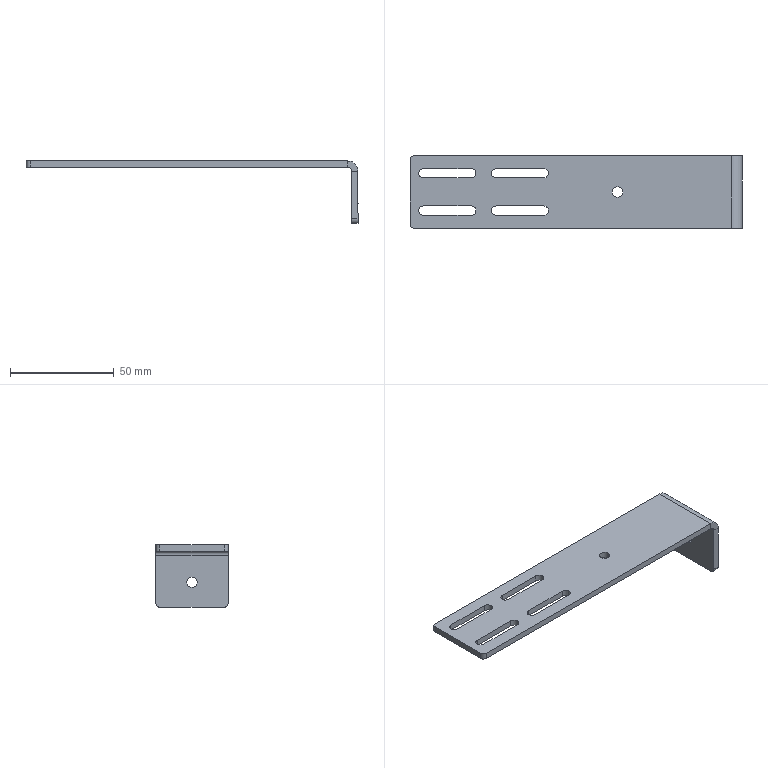Part | NX | features BREP 1 | 1 solid | 42 faces | box 160 x 35 x 30 mm | volume 17916 mm3 | cylinder 22 | plane 20 | commonest cylinder face diameters 4.5 x12 4 x5 5 x4 10 x1
STEP:
#1=CARTESIAN_POINT('',(77.,0.,-15.5));
#2=VERTEX_POINT('',#1);
#3=CARTESIAN_POINT('',(80.,0.,-15.5));
#4=VERTEX_POINT('',#3);
#5=CARTESIAN_POINT('',(80.,0.,-15.5));
#6=DIRECTION('',(1.,0.,0.));
#7=VECTOR('',#6,1000.);
#8=LINE('',#5,#7);
#9=EDGE_CURVE('',#2,#4,#8,.T.);
#10=ORIENTED_EDGE('',*,*,#9,.F.);
#11=CARTESIAN_POINT('',(77.,0.,-20.5));
#12=VERTEX_POINT('',#11);
#13=CARTESIAN_POINT('',(77.,0.,-18.));
#14=DIRECTION('',(-1.,0.,0.));
#15=DIRECTION('',(0.,0.,1.));
#16=AXIS2_PLACEMENT_3D('',#13,#14,#15);
#17=CIRCLE('',#16,2.5);
#18=EDGE_CURVE('',#2,#12,#17,.T.);
#19=ORIENTED_EDGE('',*,*,#18,.T.);
#20=CARTESIAN_POINT('',(80.,0.,-20.5));
#21=VERTEX_POINT('',#20);
#22=CARTESIAN_POINT('',(80.,0.,-20.5));
#23=DIRECTION('',(1.,0.,0.));
#24=VECTOR('',#23,1000.);
#25=LINE('',#22,#24);
#26=EDGE_CURVE('',#12,#21,#25,.T.);
#27=ORIENTED_EDGE('',*,*,#26,.T.);
#28=CARTESIAN_POINT('',(80.,0.,-18.));
#29=DIRECTION('',(1.,0.,0.));
#30=DIRECTION('',(0.,0.,-1.));
#31=AXIS2_PLACEMENT_3D('',#28,#29,#30);
#32=CIRCLE('',#31,2.5);
#33=EDGE_CURVE('',#21,#4,#32,.T.);
#34=ORIENTED_EDGE('',*,*,#33,.T.);
#35=EDGE_LOOP('',(#10,#19,#27,#34));
#36=FACE_BOUND('',#35,.T.);
#37=CARTESIAN_POINT('',(80.,0.,-18.));
#38=DIRECTION('',(1.,0.,0.));
#39=DIRECTION('',(0.,0.,-1.));
#40=AXIS2_PLACEMENT_3D('',#37,#38,#39);
#41=CYLINDRICAL_SURFACE('',#40,2.5);
#42=ADVANCED_FACE('',(#36),#41,.F.);
#43=CARTESIAN_POINT('',(-80.,15.5,-3.));
#44=VERTEX_POINT('',#43);
#45=CARTESIAN_POINT('',(-78.,17.5,-3.));
#46=VERTEX_POINT('',#45);
#47=CARTESIAN_POINT('',(-78.,15.5,-3.));
#48=DIRECTION('',(0.,0.,-1.));
#49=DIRECTION('',(1.,0.,0.));
#50=AXIS2_PLACEMENT_3D('',#47,#48,#49);
#51=CIRCLE('',#50,2.);
#52=EDGE_CURVE('',#44,#46,#51,.T.);
#53=ORIENTED_EDGE('',*,*,#52,.F.);
#54=CARTESIAN_POINT('',(-80.,15.5,0.));
#55=VERTEX_POINT('',#54);
#56=CARTESIAN_POINT('',(-80.,15.5,-3.));
#57=DIRECTION('',(0.,0.,-1.));
#58=VECTOR('',#57,1000.);
#59=LINE('',#56,#58);
#60=EDGE_CURVE('',#55,#44,#59,.T.);
#61=ORIENTED_EDGE('',*,*,#60,.F.);
#62=CARTESIAN_POINT('',(-78.,17.5,0.));
#63=VERTEX_POINT('',#62);
#64=CARTESIAN_POINT('',(-78.,15.5,0.));
#65=DIRECTION('',(0.,0.,1.));
#66=DIRECTION('',(1.,0.,0.));
#67=AXIS2_PLACEMENT_3D('',#64,#65,#66);
#68=CIRCLE('',#67,2.);
#69=EDGE_CURVE('',#63,#55,#68,.T.);
#70=ORIENTED_EDGE('',*,*,#69,.F.);
#71=CARTESIAN_POINT('',(-78.,17.5,-3.));
#72=DIRECTION('',(0.,0.,1.));
#73=VECTOR('',#72,1000.);
#74=LINE('',#71,#73);
#75=EDGE_CURVE('',#46,#63,#74,.T.);
#76=ORIENTED_EDGE('',*,*,#75,.F.);
#77=EDGE_LOOP('',(#53,#61,#70,#76));
#78=FACE_BOUND('',#77,.T.);
#79=CARTESIAN_POINT('',(-78.,15.5,-3.));
#80=DIRECTION('',(0.,0.,1.));
#81=DIRECTION('',(1.,0.,0.));
#82=AXIS2_PLACEMENT_3D('',#79,#80,#81);
#83=CYLINDRICAL_SURFACE('',#82,2.);
#84=ADVANCED_FACE('',(#78),#83,.T.);
#85=CARTESIAN_POINT('',(-78.,-17.5,-3.));
#86=VERTEX_POINT('',#85);
#87=CARTESIAN_POINT('',(-80.,-15.5,-3.));
#88=VERTEX_POINT('',#87);
#89=CARTESIAN_POINT('',(-78.,-15.5,-3.));
#90=DIRECTION('',(0.,0.,-1.));
#91=DIRECTION('',(1.,0.,0.));
#92=AXIS2_PLACEMENT_3D('',#89,#90,#91);
#93=CIRCLE('',#92,2.);
#94=EDGE_CURVE('',#86,#88,#93,.T.);
#95=ORIENTED_EDGE('',*,*,#94,.F.);
#96=CARTESIAN_POINT('',(-78.,-17.5,0.));
#97=VERTEX_POINT('',#96);
#98=CARTESIAN_POINT('',(-78.,-17.5,-3.));
#99=DIRECTION('',(0.,0.,-1.));
#100=VECTOR('',#99,1000.);
#101=LINE('',#98,#100);
#102=EDGE_CURVE('',#97,#86,#101,.T.);
#103=ORIENTED_EDGE('',*,*,#102,.F.);
#104=CARTESIAN_POINT('',(-80.,-15.5,0.));
#105=VERTEX_POINT('',#104);
#106=CARTESIAN_POINT('',(-78.,-15.5,0.));
#107=DIRECTION('',(0.,0.,1.));
#108=DIRECTION('',(1.,0.,0.));
#109=AXIS2_PLACEMENT_3D('',#106,#107,#108);
#110=CIRCLE('',#109,2.);
#111=EDGE_CURVE('',#105,#97,#110,.T.);
#112=ORIENTED_EDGE('',*,*,#111,.F.);
#113=CARTESIAN_POINT('',(-80.,-15.5,-3.));
#114=DIRECTION('',(0.,0.,1.));
#115=VECTOR('',#114,1000.);
#116=LINE('',#113,#115);
#117=EDGE_CURVE('',#88,#105,#116,.T.);
#118=ORIENTED_EDGE('',*,*,#117,.F.);
#119=EDGE_LOOP('',(#95,#103,#112,#118));
#120=FACE_BOUND('',#119,.T.);
#121=CARTESIAN_POINT('',(-78.,-15.5,-3.));
#122=DIRECTION('',(0.,0.,1.));
#123=DIRECTION('',(1.,0.,0.));
#124=AXIS2_PLACEMENT_3D('',#121,#122,#123);
#125=CYLINDRICAL_SURFACE('',#124,2.);
#126=ADVANCED_FACE('',(#120),#125,.T.);
#127=CARTESIAN_POINT('',(80.,15.5,-30.));
#128=VERTEX_POINT('',#127);
#129=CARTESIAN_POINT('',(80.,17.5,-28.));
#130=VERTEX_POINT('',#129);
#131=CARTESIAN_POINT('',(80.,15.5,-28.));
#132=DIRECTION('',(1.,0.,0.));
#133=DIRECTION('',(0.,0.,1.));
#134=AXIS2_PLACEMENT_3D('',#131,#132,#133);
#135=CIRCLE('',#134,2.);
#136=EDGE_CURVE('',#128,#130,#135,.T.);
#137=ORIENTED_EDGE('',*,*,#136,.F.);
#138=CARTESIAN_POINT('',(77.,15.5,-30.));
#139=VERTEX_POINT('',#138);
#140=CARTESIAN_POINT('',(80.,15.5,-30.));
#141=DIRECTION('',(1.,0.,0.));
#142=VECTOR('',#141,1000.);
#143=LINE('',#140,#142);
#144=EDGE_CURVE('',#139,#128,#143,.T.);
#145=ORIENTED_EDGE('',*,*,#144,.F.);
#146=CARTESIAN_POINT('',(77.,17.5,-28.));
#147=VERTEX_POINT('',#146);
#148=CARTESIAN_POINT('',(77.,15.5,-28.));
#149=DIRECTION('',(-1.,0.,0.));
#150=DIRECTION('',(0.,0.,1.));
#151=AXIS2_PLACEMENT_3D('',#148,#149,#150);
#152=CIRCLE('',#151,2.);
#153=EDGE_CURVE('',#147,#139,#152,.T.);
#154=ORIENTED_EDGE('',*,*,#153,.F.);
#155=CARTESIAN_POINT('',(80.,17.5,-28.));
#156=DIRECTION('',(-1.,0.,0.));
#157=VECTOR('',#156,1000.);
#158=LINE('',#155,#157);
#159=EDGE_CURVE('',#130,#147,#158,.T.);
#160=ORIENTED_EDGE('',*,*,#159,.F.);
#161=EDGE_LOOP('',(#137,#145,#154,#160));
#162=FACE_BOUND('',#161,.T.);
#163=CARTESIAN_POINT('',(80.,15.5,-28.));
#164=DIRECTION('',(-1.,0.,0.));
#165=DIRECTION('',(0.,0.,1.));
#166=AXIS2_PLACEMENT_3D('',#163,#164,#165);
#167=CYLINDRICAL_SURFACE('',#166,2.);
#168=ADVANCED_FACE('',(#162),#167,.T.);
#169=CARTESIAN_POINT('',(80.,-17.5,-28.));
#170=VERTEX_POINT('',#169);
#171=CARTESIAN_POINT('',(80.,-15.5,-30.));
#172=VERTEX_POINT('',#171);
#173=CARTESIAN_POINT('',(80.,-15.5,-28.));
#174=DIRECTION('',(1.,0.,0.));
#175=DIRECTION('',(0.,0.,1.));
#176=AXIS2_PLACEMENT_3D('',#173,#174,#175);
#177=CIRCLE('',#176,2.);
#178=EDGE_CURVE('',#170,#172,#177,.T.);
#179=ORIENTED_EDGE('',*,*,#178,.F.);
#180=CARTESIAN_POINT('',(77.,-17.5,-28.));
#181=VERTEX_POINT('',#180);
#182=CARTESIAN_POINT('',(80.,-17.5,-28.));
#183=DIRECTION('',(1.,0.,0.));
#184=VECTOR('',#183,1000.);
#185=LINE('',#182,#184);
#186=EDGE_CURVE('',#181,#170,#185,.T.);
#187=ORIENTED_EDGE('',*,*,#186,.F.);
#188=CARTESIAN_POINT('',(77.,-15.5,-30.));
#189=VERTEX_POINT('',#188);
#190=CARTESIAN_POINT('',(77.,-15.5,-28.));
#191=DIRECTION('',(-1.,0.,0.));
#192=DIRECTION('',(0.,0.,1.));
#193=AXIS2_PLACEMENT_3D('',#190,#191,#192);
#194=CIRCLE('',#193,2.);
#195=EDGE_CURVE('',#189,#181,#194,.T.);
#196=ORIENTED_EDGE('',*,*,#195,.F.);
#197=CARTESIAN_POINT('',(80.,-15.5,-30.));
#198=DIRECTION('',(-1.,0.,0.));
#199=VECTOR('',#198,1000.);
#200=LINE('',#197,#199);
#201=EDGE_CURVE('',#172,#189,#200,.T.);
#202=ORIENTED_EDGE('',*,*,#201,.F.);
#203=EDGE_LOOP('',(#179,#187,#196,#202));
#204=FACE_BOUND('',#203,.T.);
#205=CARTESIAN_POINT('',(80.,-15.5,-28.));
#206=DIRECTION('',(-1.,0.,0.));
#207=DIRECTION('',(0.,0.,1.));
#208=AXIS2_PLACEMENT_3D('',#205,#206,#207);
#209=CYLINDRICAL_SURFACE('',#208,2.);
#210=ADVANCED_FACE('',(#204),#209,.T.);
#211=CARTESIAN_POINT('',(-15.5,11.25,0.));
#212=VERTEX_POINT('',#211);
#213=CARTESIAN_POINT('',(-38.5,11.25,0.));
#214=VERTEX_POINT('',#213);
#215=CARTESIAN_POINT('',(0.,11.25,0.));
#216=DIRECTION('',(-1.,0.,0.));
#217=VECTOR('',#216,1000.);
#218=LINE('',#215,#217);
#219=EDGE_CURVE('',#212,#214,#218,.T.);
#220=ORIENTED_EDGE('',*,*,#219,.T.);
#221=CARTESIAN_POINT('',(-38.5,11.25,-3.));
#222=VERTEX_POINT('',#221);
#223=CARTESIAN_POINT('',(-38.5,11.25,-3.));
#224=DIRECTION('',(0.,0.,-1.));
#225=VECTOR('',#224,1000.);
#226=LINE('',#223,#225);
#227=EDGE_CURVE('',#214,#222,#226,.T.);
#228=ORIENTED_EDGE('',*,*,#227,.T.);
#229=CARTESIAN_POINT('',(-15.5,11.25,-3.));
#230=VERTEX_POINT('',#229);
#231=CARTESIAN_POINT('',(-38.5,11.25,-3.));
#232=DIRECTION('',(1.,0.,0.));
#233=VECTOR('',#232,1000.);
#234=LINE('',#231,#233);
#235=EDGE_CURVE('',#222,#230,#234,.T.);
#236=ORIENTED_EDGE('',*,*,#235,.T.);
#237=CARTESIAN_POINT('',(-15.5,11.25,-3.));
#238=DIRECTION('',(0.,0.,1.));
#239=VECTOR('',#238,1000.);
#240=LINE('',#237,#239);
#241=EDGE_CURVE('',#230,#212,#240,.T.);
#242=ORIENTED_EDGE('',*,*,#241,.T.);
#243=EDGE_LOOP('',(#220,#228,#236,#242));
#244=FACE_BOUND('',#243,.T.);
#245=CARTESIAN_POINT('',(-38.5,11.25,-3.));
#246=DIRECTION('',(0.,1.,0.));
#247=DIRECTION('',(-1.,0.,0.));
#248=AXIS2_PLACEMENT_3D('',#245,#246,#247);
#249=PLANE('',#248);
#250=ADVANCED_FACE('',(#244),#249,.F.);
#251=CARTESIAN_POINT('',(-38.5,6.75,0.));
#252=VERTEX_POINT('',#251);
#253=CARTESIAN_POINT('',(-15.5,6.75,0.));
#254=VERTEX_POINT('',#253);
#255=CARTESIAN_POINT('',(0.,6.75,0.));
#256=DIRECTION('',(1.,0.,0.));
#257=VECTOR('',#256,1000.);
#258=LINE('',#255,#257);
#259=EDGE_CURVE('',#252,#254,#258,.T.);
#260=ORIENTED_EDGE('',*,*,#259,.T.);
#261=CARTESIAN_POINT('',(-15.5,6.75,-3.));
#262=VERTEX_POINT('',#261);
#263=CARTESIAN_POINT('',(-15.5,6.75,-3.));
#264=DIRECTION('',(0.,0.,-1.));
#265=VECTOR('',#264,1000.);
#266=LINE('',#263,#265);
#267=EDGE_CURVE('',#254,#262,#266,.T.);
#268=ORIENTED_EDGE('',*,*,#267,.T.);
#269=CARTESIAN_POINT('',(-38.5,6.75,-3.));
#270=VERTEX_POINT('',#269);
#271=CARTESIAN_POINT('',(-38.5,6.75,-3.));
#272=DIRECTION('',(1.,0.,0.));
#273=VECTOR('',#272,1000.);
#274=LINE('',#271,#273);
#275=EDGE_CURVE('',#270,#262,#274,.T.);
#276=ORIENTED_EDGE('',*,*,#275,.F.);
#277=CARTESIAN_POINT('',(-38.5,6.75,-3.));
#278=DIRECTION('',(0.,0.,1.));
#279=VECTOR('',#278,1000.);
#280=LINE('',#277,#279);
#281=EDGE_CURVE('',#270,#252,#280,.T.);
#282=ORIENTED_EDGE('',*,*,#281,.T.);
#283=EDGE_LOOP('',(#260,#268,#276,#282));
#284=FACE_BOUND('',#283,.T.);
#285=CARTESIAN_POINT('',(-38.5,6.75,-3.));
#286=DIRECTION('',(0.,-1.,0.));
#287=DIRECTION('',(1.,0.,0.));
#288=AXIS2_PLACEMENT_3D('',#285,#286,#287);
#289=PLANE('',#288);
#290=ADVANCED_FACE('',(#284),#289,.F.);
#291=CARTESIAN_POINT('',(-40.75,9.,0.));
#292=VERTEX_POINT('',#291);
#293=CARTESIAN_POINT('',(-40.75,9.,-3.));
#294=VERTEX_POINT('',#293);
#295=CARTESIAN_POINT('',(-40.75,9.,-3.));
#296=DIRECTION('',(0.,0.,-1.));
#297=VECTOR('',#296,1000.);
#298=LINE('',#295,#297);
#299=EDGE_CURVE('',#292,#294,#298,.T.);
#300=ORIENTED_EDGE('',*,*,#299,.F.);
#301=CARTESIAN_POINT('',(-38.5,9.,0.));
#302=DIRECTION('',(0.,0.,1.));
#303=DIRECTION('',(1.,0.,0.));
#304=AXIS2_PLACEMENT_3D('',#301,#302,#303);
#305=CIRCLE('',#304,2.25);
#306=EDGE_CURVE('',#292,#252,#305,.T.);
#307=ORIENTED_EDGE('',*,*,#306,.T.);
#308=ORIENTED_EDGE('',*,*,#281,.F.);
#309=CARTESIAN_POINT('',(-38.5,9.,-3.));
#310=DIRECTION('',(0.,0.,-1.));
#311=DIRECTION('',(-1.,0.,0.));
#312=AXIS2_PLACEMENT_3D('',#309,#310,#311);
#313=CIRCLE('',#312,2.25);
#314=EDGE_CURVE('',#270,#294,#313,.T.);
#315=ORIENTED_EDGE('',*,*,#314,.T.);
#316=EDGE_LOOP('',(#300,#307,#308,#315));
#317=FACE_BOUND('',#316,.T.);
#318=CARTESIAN_POINT('',(-38.5,9.,-3.));
#319=DIRECTION('',(0.,0.,-1.));
#320=DIRECTION('',(-1.,0.,0.));
#321=AXIS2_PLACEMENT_3D('',#318,#319,#320);
#322=CYLINDRICAL_SURFACE('',#321,2.25);
#323=ADVANCED_FACE('',(#317),#322,.F.);
#324=CARTESIAN_POINT('',(-15.5,9.,0.));
#325=DIRECTION('',(0.,0.,1.));
#326=DIRECTION('',(1.,0.,0.));
#327=AXIS2_PLACEMENT_3D('',#324,#325,#326);
#328=CIRCLE('',#327,2.25);
#329=EDGE_CURVE('',#254,#212,#328,.T.);
#330=ORIENTED_EDGE('',*,*,#329,.T.);
#331=ORIENTED_EDGE('',*,*,#241,.F.);
#332=CARTESIAN_POINT('',(-15.5,9.,-3.));
#333=DIRECTION('',(0.,0.,-1.));
#334=DIRECTION('',(-1.,0.,0.));
#335=AXIS2_PLACEMENT_3D('',#332,#333,#334);
#336=CIRCLE('',#335,2.25);
#337=EDGE_CURVE('',#230,#262,#336,.T.);
#338=ORIENTED_EDGE('',*,*,#337,.T.);
#339=ORIENTED_EDGE('',*,*,#267,.F.);
#340=EDGE_LOOP('',(#330,#331,#338,#339));
#341=FACE_BOUND('',#340,.T.);
#342=CARTESIAN_POINT('',(-15.5,9.,-3.));
#343=DIRECTION('',(0.,0.,-1.));
#344=DIRECTION('',(-1.,0.,0.));
#345=AXIS2_PLACEMENT_3D('',#342,#343,#344);
#346=CYLINDRICAL_SURFACE('',#345,2.25);
#347=ADVANCED_FACE('',(#341),#346,.F.);
#348=CARTESIAN_POINT('',(-50.5,11.25,0.));
#349=VERTEX_POINT('',#348);
#350=CARTESIAN_POINT('',(-73.5,11.25,0.));
#351=VERTEX_POINT('',#350);
#352=CARTESIAN_POINT('',(0.,11.25,0.));
#353=DIRECTION('',(-1.,0.,0.));
#354=VECTOR('',#353,1000.);
#355=LINE('',#352,#354);
#356=EDGE_CURVE('',#349,#351,#355,.T.);
#357=ORIENTED_EDGE('',*,*,#356,.T.);
#358=CARTESIAN_POINT('',(-73.5,11.25,-3.));
#359=VERTEX_POINT('',#358);
#360=CARTESIAN_POINT('',(-73.5,11.25,-3.));
#361=DIRECTION('',(0.,0.,-1.));
#362=VECTOR('',#361,1000.);
#363=LINE('',#360,#362);
#364=EDGE_CURVE('',#351,#359,#363,.T.);
#365=ORIENTED_EDGE('',*,*,#364,.T.);
#366=CARTESIAN_POINT('',(-50.5,11.25,-3.));
#367=VERTEX_POINT('',#366);
#368=CARTESIAN_POINT('',(-73.5,11.25,-3.));
#369=DIRECTION('',(1.,0.,0.));
#370=VECTOR('',#369,1000.);
#371=LINE('',#368,#370);
#372=EDGE_CURVE('',#359,#367,#371,.T.);
#373=ORIENTED_EDGE('',*,*,#372,.T.);
#374=CARTESIAN_POINT('',(-50.5,11.25,-3.));
#375=DIRECTION('',(0.,0.,1.));
#376=VECTOR('',#375,1000.);
#377=LINE('',#374,#376);
#378=EDGE_CURVE('',#367,#349,#377,.T.);
#379=ORIENTED_EDGE('',*,*,#378,.T.);
#380=EDGE_LOOP('',(#357,#365,#373,#379));
#381=FACE_BOUND('',#380,.T.);
#382=CARTESIAN_POINT('',(-73.5,11.25,-3.));
#383=DIRECTION('',(0.,1.,0.));
#384=DIRECTION('',(-1.,0.,0.));
#385=AXIS2_PLACEMENT_3D('',#382,#383,#384);
#386=PLANE('',#385);
#387=ADVANCED_FACE('',(#381),#386,.F.);
#388=CARTESIAN_POINT('',(-73.5,6.75,0.));
#389=VERTEX_POINT('',#388);
#390=CARTESIAN_POINT('',(-50.5,6.75,0.));
#391=VERTEX_POINT('',#390);
#392=CARTESIAN_POINT('',(0.,6.75,0.));
#393=DIRECTION('',(1.,0.,0.));
#394=VECTOR('',#393,1000.);
#395=LINE('',#392,#394);
#396=EDGE_CURVE('',#389,#391,#395,.T.);
#397=ORIENTED_EDGE('',*,*,#396,.T.);
#398=CARTESIAN_POINT('',(-50.5,6.75,-3.));
#399=VERTEX_POINT('',#398);
#400=CARTESIAN_POINT('',(-50.5,6.75,-3.));
#401=DIRECTION('',(0.,0.,-1.));
#402=VECTOR('',#401,1000.);
#403=LINE('',#400,#402);
#404=EDGE_CURVE('',#391,#399,#403,.T.);
#405=ORIENTED_EDGE('',*,*,#404,.T.);
#406=CARTESIAN_POINT('',(-73.5,6.75,-3.));
#407=VERTEX_POINT('',#406);
#408=CARTESIAN_POINT('',(-73.5,6.75,-3.));
#409=DIRECTION('',(1.,0.,0.));
#410=VECTOR('',#409,1000.);
#411=LINE('',#408,#410);
#412=EDGE_CURVE('',#407,#399,#411,.T.);
#413=ORIENTED_EDGE('',*,*,#412,.F.);
#414=CARTESIAN_POINT('',(-73.5,6.75,-3.));
#415=DIRECTION('',(0.,0.,1.));
#416=VECTOR('',#415,1000.);
#417=LINE('',#414,#416);
#418=EDGE_CURVE('',#407,#389,#417,.T.);
#419=ORIENTED_EDGE('',*,*,#418,.T.);
#420=EDGE_LOOP('',(#397,#405,#413,#419));
#421=FACE_BOUND('',#420,.T.);
#422=CARTESIAN_POINT('',(-73.5,6.75,-3.));
#423=DIRECTION('',(0.,-1.,0.));
#424=DIRECTION('',(1.,0.,0.));
#425=AXIS2_PLACEMENT_3D('',#422,#423,#424);
#426=PLANE('',#425);
#427=ADVANCED_FACE('',(#421),#426,.F.);
#428=CARTESIAN_POINT('',(-75.75,9.,0.));
#429=VERTEX_POINT('',#428);
#430=CARTESIAN_POINT('',(-75.75,9.,-3.));
#431=VERTEX_POINT('',#430);
#432=CARTESIAN_POINT('',(-75.75,9.,-3.));
#433=DIRECTION('',(0.,0.,-1.));
#434=VECTOR('',#433,1000.);
#435=LINE('',#432,#434);
#436=EDGE_CURVE('',#429,#431,#435,.T.);
#437=ORIENTED_EDGE('',*,*,#436,.F.);
#438=CARTESIAN_POINT('',(-73.5,9.,0.));
#439=DIRECTION('',(0.,0.,1.));
#440=DIRECTION('',(1.,0.,0.));
#441=AXIS2_PLACEMENT_3D('',#438,#439,#440);
#442=CIRCLE('',#441,2.25);
#443=EDGE_CURVE('',#429,#389,#442,.T.);
#444=ORIENTED_EDGE('',*,*,#443,.T.);
#445=ORIENTED_EDGE('',*,*,#418,.F.);
#446=CARTESIAN_POINT('',(-73.5,9.,-3.));
#447=DIRECTION('',(0.,0.,-1.));
#448=DIRECTION('',(-1.,0.,0.));
#449=AXIS2_PLACEMENT_3D('',#446,#447,#448);
#450=CIRCLE('',#449,2.25);
#451=EDGE_CURVE('',#407,#431,#450,.T.);
#452=ORIENTED_EDGE('',*,*,#451,.T.);
#453=EDGE_LOOP('',(#437,#444,#445,#452));
#454=FACE_BOUND('',#453,.T.);
#455=CARTESIAN_POINT('',(-73.5,9.,-3.));
#456=DIRECTION('',(0.,0.,-1.));
#457=DIRECTION('',(-1.,0.,0.));
#458=AXIS2_PLACEMENT_3D('',#455,#456,#457);
#459=CYLINDRICAL_SURFACE('',#458,2.25);
#460=ADVANCED_FACE('',(#454),#459,.F.);
#461=CARTESIAN_POINT('',(-50.5,9.,0.));
#462=DIRECTION('',(0.,0.,1.));
#463=DIRECTION('',(1.,0.,0.));
#464=AXIS2_PLACEMENT_3D('',#461,#462,#463);
#465=CIRCLE('',#464,2.25);
#466=EDGE_CURVE('',#391,#349,#465,.T.);
#467=ORIENTED_EDGE('',*,*,#466,.T.);
#468=ORIENTED_EDGE('',*,*,#378,.F.);
#469=CARTESIAN_POINT('',(-50.5,9.,-3.));
#470=DIRECTION('',(0.,0.,-1.));
#471=DIRECTION('',(-1.,0.,0.));
#472=AXIS2_PLACEMENT_3D('',#469,#470,#471);
#473=CIRCLE('',#472,2.25);
#474=EDGE_CURVE('',#367,#399,#473,.T.);
#475=ORIENTED_EDGE('',*,*,#474,.T.);
#476=ORIENTED_EDGE('',*,*,#404,.F.);
#477=EDGE_LOOP('',(#467,#468,#475,#476));
#478=FACE_BOUND('',#477,.T.);
#479=CARTESIAN_POINT('',(-50.5,9.,-3.));
#480=DIRECTION('',(0.,0.,-1.));
#481=DIRECTION('',(-1.,0.,0.));
#482=AXIS2_PLACEMENT_3D('',#479,#480,#481);
#483=CYLINDRICAL_SURFACE('',#482,2.25);
#484=ADVANCED_FACE('',(#478),#483,.F.);
#485=CARTESIAN_POINT('',(-15.5,-6.75,0.));
#486=VERTEX_POINT('',#485);
#487=CARTESIAN_POINT('',(-38.5,-6.75,0.));
#488=VERTEX_POINT('',#487);
#489=CARTESIAN_POINT('',(0.,-6.75,0.));
#490=DIRECTION('',(-1.,0.,0.));
#491=VECTOR('',#490,1000.);
#492=LINE('',#489,#491);
#493=EDGE_CURVE('',#486,#488,#492,.T.);
#494=ORIENTED_EDGE('',*,*,#493,.T.);
#495=CARTESIAN_POINT('',(-38.5,-6.75,-3.));
#496=VERTEX_POINT('',#495);
#497=CARTESIAN_POINT('',(-38.5,-6.75,-3.));
#498=DIRECTION('',(0.,0.,-1.));
#499=VECTOR('',#498,1000.);
#500=LINE('',#497,#499);
#501=EDGE_CURVE('',#488,#496,#500,.T.);
#502=ORIENTED_EDGE('',*,*,#501,.T.);
#503=CARTESIAN_POINT('',(-15.5,-6.75,-3.));
#504=VERTEX_POINT('',#503);
#505=CARTESIAN_POINT('',(-38.5,-6.75,-3.));
#506=DIRECTION('',(1.,0.,0.));
#507=VECTOR('',#506,1000.);
#508=LINE('',#505,#507);
#509=EDGE_CURVE('',#496,#504,#508,.T.);
#510=ORIENTED_EDGE('',*,*,#509,.T.);
#511=CARTESIAN_POINT('',(-15.5,-6.75,-3.));
#512=DIRECTION('',(0.,0.,1.));
#513=VECTOR('',#512,1000.);
#514=LINE('',#511,#513);
#515=EDGE_CURVE('',#504,#486,#514,.T.);
#516=ORIENTED_EDGE('',*,*,#515,.T.);
#517=EDGE_LOOP('',(#494,#502,#510,#516));
#518=FACE_BOUND('',#517,.T.);
#519=CARTESIAN_POINT('',(-38.5,-6.75,-3.));
#520=DIRECTION('',(0.,1.,0.));
#521=DIRECTION('',(-1.,0.,0.));
#522=AXIS2_PLACEMENT_3D('',#519,#520,#521);
#523=PLANE('',#522);
#524=ADVANCED_FACE('',(#518),#523,.F.);
#525=CARTESIAN_POINT('',(-38.5,-11.25,0.));
#526=VERTEX_POINT('',#525);
#527=CARTESIAN_POINT('',(-15.5,-11.25,0.));
#528=VERTEX_POINT('',#527);
#529=CARTESIAN_POINT('',(0.,-11.25,0.));
#530=DIRECTION('',(1.,0.,0.));
#531=VECTOR('',#530,1000.);
#532=LINE('',#529,#531);
#533=EDGE_CURVE('',#526,#528,#532,.T.);
#534=ORIENTED_EDGE('',*,*,#533,.T.);
#535=CARTESIAN_POINT('',(-15.5,-11.25,-3.));
#536=VERTEX_POINT('',#535);
#537=CARTESIAN_POINT('',(-15.5,-11.25,-3.));
#538=DIRECTION('',(0.,0.,-1.));
#539=VECTOR('',#538,1000.);
#540=LINE('',#537,#539);
#541=EDGE_CURVE('',#528,#536,#540,.T.);
#542=ORIENTED_EDGE('',*,*,#541,.T.);
#543=CARTESIAN_POINT('',(-38.5,-11.25,-3.));
#544=VERTEX_POINT('',#543);
#545=CARTESIAN_POINT('',(-38.5,-11.25,-3.));
#546=DIRECTION('',(1.,0.,0.));
#547=VECTOR('',#546,1000.);
#548=LINE('',#545,#547);
#549=EDGE_CURVE('',#544,#536,#548,.T.);
#550=ORIENTED_EDGE('',*,*,#549,.F.);
#551=CARTESIAN_POINT('',(-38.5,-11.25,-3.));
#552=DIRECTION('',(0.,0.,1.));
#553=VECTOR('',#552,1000.);
#554=LINE('',#551,#553);
#555=EDGE_CURVE('',#544,#526,#554,.T.);
#556=ORIENTED_EDGE('',*,*,#555,.T.);
#557=EDGE_LOOP('',(#534,#542,#550,#556));
#558=FACE_BOUND('',#557,.T.);
#559=CARTESIAN_POINT('',(-38.5,-11.25,-3.));
#560=DIRECTION('',(0.,-1.,0.));
#561=DIRECTION('',(1.,0.,0.));
#562=AXIS2_PLACEMENT_3D('',#559,#560,#561);
#563=PLANE('',#562);
#564=ADVANCED_FACE('',(#558),#563,.F.);
#565=CARTESIAN_POINT('',(-40.75,-9.,0.));
#566=VERTEX_POINT('',#565);
#567=CARTESIAN_POINT('',(-40.75,-9.,-3.));
#568=VERTEX_POINT('',#567);
#569=CARTESIAN_POINT('',(-40.75,-9.,-3.));
#570=DIRECTION('',(0.,0.,-1.));
#571=VECTOR('',#570,1000.);
#572=LINE('',#569,#571);
#573=EDGE_CURVE('',#566,#568,#572,.T.);
#574=ORIENTED_EDGE('',*,*,#573,.F.);
#575=CARTESIAN_POINT('',(-38.5,-9.,0.));
#576=DIRECTION('',(0.,0.,1.));
#577=DIRECTION('',(1.,0.,0.));
#578=AXIS2_PLACEMENT_3D('',#575,#576,#577);
#579=CIRCLE('',#578,2.25);
#580=EDGE_CURVE('',#566,#526,#579,.T.);
#581=ORIENTED_EDGE('',*,*,#580,.T.);
#582=ORIENTED_EDGE('',*,*,#555,.F.);
#583=CARTESIAN_POINT('',(-38.5,-9.,-3.));
#584=DIRECTION('',(0.,0.,-1.));
#585=DIRECTION('',(-1.,0.,0.));
#586=AXIS2_PLACEMENT_3D('',#583,#584,#585);
#587=CIRCLE('',#586,2.25);
#588=EDGE_CURVE('',#544,#568,#587,.T.);
#589=ORIENTED_EDGE('',*,*,#588,.T.);
#590=EDGE_LOOP('',(#574,#581,#582,#589));
#591=FACE_BOUND('',#590,.T.);
#592=CARTESIAN_POINT('',(-38.5,-9.,-3.));
#593=DIRECTION('',(0.,0.,-1.));
#594=DIRECTION('',(-1.,0.,0.));
#595=AXIS2_PLACEMENT_3D('',#592,#593,#594);
#596=CYLINDRICAL_SURFACE('',#595,2.25);
#597=ADVANCED_FACE('',(#591),#596,.F.);
#598=CARTESIAN_POINT('',(-15.5,-9.,0.));
#599=DIRECTION('',(0.,0.,1.));
#600=DIRECTION('',(1.,0.,0.));
#601=AXIS2_PLACEMENT_3D('',#598,#599,#600);
#602=CIRCLE('',#601,2.25);
#603=EDGE_CURVE('',#528,#486,#602,.T.);
#604=ORIENTED_EDGE('',*,*,#603,.T.);
#605=ORIENTED_EDGE('',*,*,#515,.F.);
#606=CARTESIAN_POINT('',(-15.5,-9.,-3.));
#607=DIRECTION('',(0.,0.,-1.));
#608=DIRECTION('',(-1.,0.,0.));
#609=AXIS2_PLACEMENT_3D('',#606,#607,#608);
#610=CIRCLE('',#609,2.25);
#611=EDGE_CURVE('',#504,#536,#610,.T.);
#612=ORIENTED_EDGE('',*,*,#611,.T.);
#613=ORIENTED_EDGE('',*,*,#541,.F.);
#614=EDGE_LOOP('',(#604,#605,#612,#613));
#615=FACE_BOUND('',#614,.T.);
#616=CARTESIAN_POINT('',(-15.5,-9.,-3.));
#617=DIRECTION('',(0.,0.,-1.));
#618=DIRECTION('',(-1.,0.,0.));
#619=AXIS2_PLACEMENT_3D('',#616,#617,#618);
#620=CYLINDRICAL_SURFACE('',#619,2.25);
#621=ADVANCED_FACE('',(#615),#620,.F.);
#622=CARTESIAN_POINT('',(-50.5,-6.75,0.));
#623=VERTEX_POINT('',#622);
#624=CARTESIAN_POINT('',(-73.5,-6.75,0.));
#625=VERTEX_POINT('',#624);
#626=CARTESIAN_POINT('',(0.,-6.75,0.));
#627=DIRECTION('',(-1.,0.,0.));
#628=VECTOR('',#627,1000.);
#629=LINE('',#626,#628);
#630=EDGE_CURVE('',#623,#625,#629,.T.);
#631=ORIENTED_EDGE('',*,*,#630,.T.);
#632=CARTESIAN_POINT('',(-73.5,-6.75,-3.));
#633=VERTEX_POINT('',#632);
#634=CARTESIAN_POINT('',(-73.5,-6.75,-3.));
#635=DIRECTION('',(0.,0.,-1.));
#636=VECTOR('',#635,1000.);
#637=LINE('',#634,#636);
#638=EDGE_CURVE('',#625,#633,#637,.T.);
#639=ORIENTED_EDGE('',*,*,#638,.T.);
#640=CARTESIAN_POINT('',(-50.5,-6.75,-3.));
#641=VERTEX_POINT('',#640);
#642=CARTESIAN_POINT('',(-73.5,-6.75,-3.));
#643=DIRECTION('',(1.,0.,0.));
#644=VECTOR('',#643,1000.);
#645=LINE('',#642,#644);
#646=EDGE_CURVE('',#633,#641,#645,.T.);
#647=ORIENTED_EDGE('',*,*,#646,.T.);
#648=CARTESIAN_POINT('',(-50.5,-6.75,-3.));
#649=DIRECTION('',(0.,0.,1.));
#650=VECTOR('',#649,1000.);
#651=LINE('',#648,#650);
#652=EDGE_CURVE('',#641,#623,#651,.T.);
#653=ORIENTED_EDGE('',*,*,#652,.T.);
#654=EDGE_LOOP('',(#631,#639,#647,#653));
#655=FACE_BOUND('',#654,.T.);
#656=CARTESIAN_POINT('',(-73.5,-6.75,-3.));
#657=DIRECTION('',(0.,1.,0.));
#658=DIRECTION('',(-1.,0.,0.));
#659=AXIS2_PLACEMENT_3D('',#656,#657,#658);
#660=PLANE('',#659);
#661=ADVANCED_FACE('',(#655),#660,.F.);
#662=CARTESIAN_POINT('',(-73.5,-11.25,0.));
#663=VERTEX_POINT('',#662);
#664=CARTESIAN_POINT('',(-50.5,-11.25,0.));
#665=VERTEX_POINT('',#664);
#666=CARTESIAN_POINT('',(0.,-11.25,0.));
#667=DIRECTION('',(1.,0.,0.));
#668=VECTOR('',#667,1000.);
#669=LINE('',#666,#668);
#670=EDGE_CURVE('',#663,#665,#669,.T.);
#671=ORIENTED_EDGE('',*,*,#670,.T.);
#672=CARTESIAN_POINT('',(-50.5,-11.25,-3.));
#673=VERTEX_POINT('',#672);
#674=CARTESIAN_POINT('',(-50.5,-11.25,-3.));
#675=DIRECTION('',(0.,0.,-1.));
#676=VECTOR('',#675,1000.);
#677=LINE('',#674,#676);
#678=EDGE_CURVE('',#665,#673,#677,.T.);
#679=ORIENTED_EDGE('',*,*,#678,.T.);
#680=CARTESIAN_POINT('',(-73.5,-11.25,-3.));
#681=VERTEX_POINT('',#680);
#682=CARTESIAN_POINT('',(-73.5,-11.25,-3.));
#683=DIRECTION('',(1.,0.,0.));
#684=VECTOR('',#683,1000.);
#685=LINE('',#682,#684);
#686=EDGE_CURVE('',#681,#673,#685,.T.);
#687=ORIENTED_EDGE('',*,*,#686,.F.);
#688=CARTESIAN_POINT('',(-73.5,-11.25,-3.));
#689=DIRECTION('',(0.,0.,1.));
#690=VECTOR('',#689,1000.);
#691=LINE('',#688,#690);
#692=EDGE_CURVE('',#681,#663,#691,.T.);
#693=ORIENTED_EDGE('',*,*,#692,.T.);
#694=EDGE_LOOP('',(#671,#679,#687,#693));
#695=FACE_BOUND('',#694,.T.);
#696=CARTESIAN_POINT('',(-73.5,-11.25,-3.));
#697=DIRECTION('',(0.,-1.,0.));
#698=DIRECTION('',(1.,0.,0.));
#699=AXIS2_PLACEMENT_3D('',#696,#697,#698);
#700=PLANE('',#699);
#701=ADVANCED_FACE('',(#695),#700,.F.);
#702=CARTESIAN_POINT('',(-75.75,-9.,0.));
#703=VERTEX_POINT('',#702);
#704=CARTESIAN_POINT('',(-75.75,-9.,-3.));
#705=VERTEX_POINT('',#704);
#706=CARTESIAN_POINT('',(-75.75,-9.,-3.));
#707=DIRECTION('',(0.,0.,-1.));
#708=VECTOR('',#707,1000.);
#709=LINE('',#706,#708);
#710=EDGE_CURVE('',#703,#705,#709,.T.);
#711=ORIENTED_EDGE('',*,*,#710,.F.);
#712=CARTESIAN_POINT('',(-73.5,-9.,0.));
#713=DIRECTION('',(0.,0.,1.));
#714=DIRECTION('',(1.,0.,0.));
#715=AXIS2_PLACEMENT_3D('',#712,#713,#714);
#716=CIRCLE('',#715,2.25);
#717=EDGE_CURVE('',#703,#663,#716,.T.);
#718=ORIENTED_EDGE('',*,*,#717,.T.);
#719=ORIENTED_EDGE('',*,*,#692,.F.);
#720=CARTESIAN_POINT('',(-73.5,-9.,-3.));
#721=DIRECTION('',(0.,0.,-1.));
#722=DIRECTION('',(-1.,0.,0.));
#723=AXIS2_PLACEMENT_3D('',#720,#721,#722);
#724=CIRCLE('',#723,2.25);
#725=EDGE_CURVE('',#681,#705,#724,.T.);
#726=ORIENTED_EDGE('',*,*,#725,.T.);
#727=EDGE_LOOP('',(#711,#718,#719,#726));
#728=FACE_BOUND('',#727,.T.);
#729=CARTESIAN_POINT('',(-73.5,-9.,-3.));
#730=DIRECTION('',(0.,0.,-1.));
#731=DIRECTION('',(-1.,0.,0.));
#732=AXIS2_PLACEMENT_3D('',#729,#730,#731);
#733=CYLINDRICAL_SURFACE('',#732,2.25);
#734=ADVANCED_FACE('',(#728),#733,.F.);
#735=CARTESIAN_POINT('',(-50.5,-9.,0.));
#736=DIRECTION('',(0.,0.,1.));
#737=DIRECTION('',(1.,0.,0.));
#738=AXIS2_PLACEMENT_3D('',#735,#736,#737);
#739=CIRCLE('',#738,2.25);
#740=EDGE_CURVE('',#665,#623,#739,.T.);
#741=ORIENTED_EDGE('',*,*,#740,.T.);
#742=ORIENTED_EDGE('',*,*,#652,.F.);
#743=CARTESIAN_POINT('',(-50.5,-9.,-3.));
#744=DIRECTION('',(0.,0.,-1.));
#745=DIRECTION('',(-1.,0.,0.));
#746=AXIS2_PLACEMENT_3D('',#743,#744,#745);
#747=CIRCLE('',#746,2.25);
#748=EDGE_CURVE('',#641,#673,#747,.T.);
#749=ORIENTED_EDGE('',*,*,#748,.T.);
#750=ORIENTED_EDGE('',*,*,#678,.F.);
#751=EDGE_LOOP('',(#741,#742,#749,#750));
#752=FACE_BOUND('',#751,.T.);
#753=CARTESIAN_POINT('',(-50.5,-9.,-3.));
#754=DIRECTION('',(0.,0.,-1.));
#755=DIRECTION('',(-1.,0.,0.));
#756=AXIS2_PLACEMENT_3D('',#753,#754,#755);
#757=CYLINDRICAL_SURFACE('',#756,2.25);
#758=ADVANCED_FACE('',(#752),#757,.F.);
#759=CARTESIAN_POINT('',(22.5,0.,0.));
#760=VERTEX_POINT('',#759);
#761=CARTESIAN_POINT('',(22.5,0.,-3.));
#762=VERTEX_POINT('',#761);
#763=CARTESIAN_POINT('',(22.5,0.,-3.));
#764=DIRECTION('',(0.,0.,-1.));
#765=VECTOR('',#764,1000.);
#766=LINE('',#763,#765);
#767=EDGE_CURVE('',#760,#762,#766,.T.);
#768=ORIENTED_EDGE('',*,*,#767,.F.);
#769=CARTESIAN_POINT('',(17.5,0.,0.));
#770=VERTEX_POINT('',#769);
#771=CARTESIAN_POINT('',(20.,0.,0.));
#772=DIRECTION('',(0.,0.,1.));
#773=DIRECTION('',(1.,0.,0.));
#774=AXIS2_PLACEMENT_3D('',#771,#772,#773);
#775=CIRCLE('',#774,2.5);
#776=EDGE_CURVE('',#760,#770,#775,.T.);
#777=ORIENTED_EDGE('',*,*,#776,.T.);
#778=CARTESIAN_POINT('',(17.5,0.,-3.));
#779=VERTEX_POINT('',#778);
#780=CARTESIAN_POINT('',(17.5,0.,-3.));
#781=DIRECTION('',(0.,0.,-1.));
#782=VECTOR('',#781,1000.);
#783=LINE('',#780,#782);
#784=EDGE_CURVE('',#770,#779,#783,.T.);
#785=ORIENTED_EDGE('',*,*,#784,.T.);
#786=CARTESIAN_POINT('',(20.,0.,-3.));
#787=DIRECTION('',(0.,0.,-1.));
#788=DIRECTION('',(-1.,0.,0.));
#789=AXIS2_PLACEMENT_3D('',#786,#787,#788);
#790=CIRCLE('',#789,2.5);
#791=EDGE_CURVE('',#779,#762,#790,.T.);
#792=ORIENTED_EDGE('',*,*,#791,.T.);
#793=EDGE_LOOP('',(#768,#777,#785,#792));
#794=FACE_BOUND('',#793,.T.);
#795=CARTESIAN_POINT('',(20.,0.,-3.));
#796=DIRECTION('',(0.,0.,-1.));
#797=DIRECTION('',(-1.,0.,0.));
#798=AXIS2_PLACEMENT_3D('',#795,#796,#797);
#799=CYLINDRICAL_SURFACE('',#798,2.5);
#800=ADVANCED_FACE('',(#794),#799,.F.);
#801=CARTESIAN_POINT('',(80.,0.,-30.));
#802=DIRECTION('',(0.,1.,0.));
#803=VECTOR('',#802,1000.);
#804=LINE('',#801,#803);
#805=EDGE_CURVE('',#172,#128,#804,.T.);
#806=ORIENTED_EDGE('',*,*,#805,.F.);
#807=ORIENTED_EDGE('',*,*,#201,.T.);
#808=CARTESIAN_POINT('',(77.,17.5,-30.));
#809=DIRECTION('',(0.,1.,0.));
#810=VECTOR('',#809,1000.);
#811=LINE('',#808,#810);
#812=EDGE_CURVE('',#189,#139,#811,.T.);
#813=ORIENTED_EDGE('',*,*,#812,.T.);
#814=ORIENTED_EDGE('',*,*,#144,.T.);
#815=EDGE_LOOP('',(#806,#807,#813,#814));
#816=FACE_BOUND('',#815,.T.);
#817=CARTESIAN_POINT('',(80.,17.5,-30.));
#818=DIRECTION('',(0.,0.,1.));
#819=DIRECTION('',(1.,0.,0.));
#820=AXIS2_PLACEMENT_3D('',#817,#818,#819);
#821=PLANE('',#820);
#822=ADVANCED_FACE('',(#816),#821,.F.);
#823=ORIENTED_EDGE('',*,*,#812,.F.);
#824=ORIENTED_EDGE('',*,*,#195,.T.);
#825=CARTESIAN_POINT('',(77.,-17.5,-5.));
#826=VERTEX_POINT('',#825);
#827=CARTESIAN_POINT('',(77.,-17.5,-30.));
#828=DIRECTION('',(0.,0.,-1.));
#829=VECTOR('',#828,1000.);
#830=LINE('',#827,#829);
#831=EDGE_CURVE('',#826,#181,#830,.T.);
#832=ORIENTED_EDGE('',*,*,#831,.F.);
#833=CARTESIAN_POINT('',(77.,17.5,-5.));
#834=VERTEX_POINT('',#833);
#835=CARTESIAN_POINT('',(77.,17.5,-5.));
#836=DIRECTION('',(0.,-1.,0.));
#837=VECTOR('',#836,1000.);
#838=LINE('',#835,#837);
#839=EDGE_CURVE('',#834,#826,#838,.T.);
#840=ORIENTED_EDGE('',*,*,#839,.F.);
#841=CARTESIAN_POINT('',(77.,17.5,-3.));
#842=DIRECTION('',(0.,0.,1.));
#843=VECTOR('',#842,1000.);
#844=LINE('',#841,#843);
#845=EDGE_CURVE('',#147,#834,#844,.T.);
#846=ORIENTED_EDGE('',*,*,#845,.F.);
#847=ORIENTED_EDGE('',*,*,#153,.T.);
#848=EDGE_LOOP('',(#823,#824,#832,#840,#846,#847));
#849=FACE_BOUND('',#848,.T.);
#850=CARTESIAN_POINT('',(77.,0.,-18.));
#851=DIRECTION('',(-1.,0.,0.));
#852=DIRECTION('',(0.,0.,1.));
#853=AXIS2_PLACEMENT_3D('',#850,#851,#852);
#854=CIRCLE('',#853,2.5);
#855=EDGE_CURVE('',#12,#2,#854,.T.);
#856=ORIENTED_EDGE('',*,*,#855,.F.);
#857=ORIENTED_EDGE('',*,*,#18,.F.);
#858=EDGE_LOOP('',(#856,#857));
#859=FACE_BOUND('',#858,.T.);
#860=CARTESIAN_POINT('',(77.,0.,0.));
#861=DIRECTION('',(-1.,0.,0.));
#862=DIRECTION('',(0.,0.,1.));
#863=AXIS2_PLACEMENT_3D('',#860,#861,#862);
#864=PLANE('',#863);
#865=ADVANCED_FACE('',(#849,#859),#864,.T.);
#866=CARTESIAN_POINT('',(80.,17.5,-5.));
#867=VERTEX_POINT('',#866);
#868=CARTESIAN_POINT('',(80.,17.5,0.));
#869=DIRECTION('',(0.,0.,1.));
#870=VECTOR('',#869,1000.);
#871=LINE('',#868,#870);
#872=EDGE_CURVE('',#130,#867,#871,.T.);
#873=ORIENTED_EDGE('',*,*,#872,.F.);
#874=ORIENTED_EDGE('',*,*,#159,.T.);
#875=ORIENTED_EDGE('',*,*,#845,.T.);
#876=CARTESIAN_POINT('',(80.,17.5,-5.));
#877=DIRECTION('',(1.,0.,0.));
#878=VECTOR('',#877,1000.);
#879=LINE('',#876,#878);
#880=EDGE_CURVE('',#834,#867,#879,.T.);
#881=ORIENTED_EDGE('',*,*,#880,.T.);
#882=EDGE_LOOP('',(#873,#874,#875,#881));
#883=FACE_BOUND('',#882,.T.);
#884=CARTESIAN_POINT('',(80.,17.5,-3.));
#885=DIRECTION('',(0.,-1.,0.));
#886=DIRECTION('',(0.,0.,-1.));
#887=AXIS2_PLACEMENT_3D('',#884,#885,#886);
#888=PLANE('',#887);
#889=ADVANCED_FACE('',(#883),#888,.F.);
#890=ORIENTED_EDGE('',*,*,#831,.T.);
#891=ORIENTED_EDGE('',*,*,#186,.T.);
#892=CARTESIAN_POINT('',(80.,-17.5,-5.));
#893=VERTEX_POINT('',#892);
#894=CARTESIAN_POINT('',(80.,-17.5,0.));
#895=DIRECTION('',(0.,0.,-1.));
#896=VECTOR('',#895,1000.);
#897=LINE('',#894,#896);
#898=EDGE_CURVE('',#893,#170,#897,.T.);
#899=ORIENTED_EDGE('',*,*,#898,.F.);
#900=CARTESIAN_POINT('',(77.,-17.5,-5.));
#901=DIRECTION('',(1.,0.,0.));
#902=VECTOR('',#901,1000.);
#903=LINE('',#900,#902);
#904=EDGE_CURVE('',#826,#893,#903,.T.);
#905=ORIENTED_EDGE('',*,*,#904,.F.);
#906=EDGE_LOOP('',(#890,#891,#899,#905));
#907=FACE_BOUND('',#906,.T.);
#908=CARTESIAN_POINT('',(80.,-17.5,-30.));
#909=DIRECTION('',(0.,1.,0.));
#910=DIRECTION('',(0.,0.,1.));
#911=AXIS2_PLACEMENT_3D('',#908,#909,#910);
#912=PLANE('',#911);
#913=ADVANCED_FACE('',(#907),#912,.F.);
#914=CARTESIAN_POINT('',(75.,-17.5,-3.));
#915=VERTEX_POINT('',#914);
#916=CARTESIAN_POINT('',(75.,17.5,-3.));
#917=VERTEX_POINT('',#916);
#918=CARTESIAN_POINT('',(75.,-17.5,-3.));
#919=DIRECTION('',(0.,1.,0.));
#920=VECTOR('',#919,1000.);
#921=LINE('',#918,#920);
#922=EDGE_CURVE('',#915,#917,#921,.T.);
#923=ORIENTED_EDGE('',*,*,#922,.T.);
#924=CARTESIAN_POINT('',(75.,17.5,-5.));
#925=DIRECTION('',(0.,1.,0.));
#926=DIRECTION('',(0.,0.,-1.));
#927=AXIS2_PLACEMENT_3D('',#924,#925,#926);
#928=CIRCLE('',#927,2.);
#929=EDGE_CURVE('',#917,#834,#928,.T.);
#930=ORIENTED_EDGE('',*,*,#929,.T.);
#931=ORIENTED_EDGE('',*,*,#839,.T.);
#932=CARTESIAN_POINT('',(75.,-17.5,-5.));
#933=DIRECTION('',(0.,-1.,0.));
#934=DIRECTION('',(0.,0.,-1.));
#935=AXIS2_PLACEMENT_3D('',#932,#933,#934);
#936=CIRCLE('',#935,2.);
#937=EDGE_CURVE('',#826,#915,#936,.T.);
#938=ORIENTED_EDGE('',*,*,#937,.T.);
#939=EDGE_LOOP('',(#923,#930,#931,#938));
#940=FACE_BOUND('',#939,.T.);
#941=CARTESIAN_POINT('',(75.,-17.5,-5.));
#942=DIRECTION('',(0.,-1.,0.));
#943=DIRECTION('',(1.,0.,0.));
#944=AXIS2_PLACEMENT_3D('',#941,#942,#943);
#945=CYLINDRICAL_SURFACE('',#944,2.);
#946=ADVANCED_FACE('',(#940),#945,.F.);
#947=CARTESIAN_POINT('',(75.,-17.5,0.));
#948=VERTEX_POINT('',#947);
#949=CARTESIAN_POINT('',(75.,17.5,0.));
#950=VERTEX_POINT('',#949);
#951=CARTESIAN_POINT('',(75.,-17.5,0.));
#952=DIRECTION('',(0.,1.,0.));
#953=VECTOR('',#952,1000.);
#954=LINE('',#951,#953);
#955=EDGE_CURVE('',#948,#950,#954,.T.);
#956=ORIENTED_EDGE('',*,*,#955,.F.);
#957=CARTESIAN_POINT('',(75.,-17.5,-5.));
#958=DIRECTION('',(0.,-1.,0.));
#959=DIRECTION('',(0.,0.,-1.));
#960=AXIS2_PLACEMENT_3D('',#957,#958,#959);
#961=CIRCLE('',#960,5.);
#962=EDGE_CURVE('',#893,#948,#961,.T.);
#963=ORIENTED_EDGE('',*,*,#962,.F.);
#964=CARTESIAN_POINT('',(80.,17.5,-5.));
#965=DIRECTION('',(0.,1.,0.));
#966=VECTOR('',#965,1000.);
#967=LINE('',#964,#966);
#968=EDGE_CURVE('',#893,#867,#967,.T.);
#969=ORIENTED_EDGE('',*,*,#968,.T.);
#970=CARTESIAN_POINT('',(75.,17.5,-5.));
#971=DIRECTION('',(0.,1.,0.));
#972=DIRECTION('',(0.,0.,-1.));
#973=AXIS2_PLACEMENT_3D('',#970,#971,#972);
#974=CIRCLE('',#973,5.);
#975=EDGE_CURVE('',#950,#867,#974,.T.);
#976=ORIENTED_EDGE('',*,*,#975,.F.);
#977=EDGE_LOOP('',(#956,#963,#969,#976));
#978=FACE_BOUND('',#977,.T.);
#979=CARTESIAN_POINT('',(75.,-17.5,-5.));
#980=DIRECTION('',(0.,-1.,0.));
#981=DIRECTION('',(1.,0.,0.));
#982=AXIS2_PLACEMENT_3D('',#979,#980,#981);
#983=CYLINDRICAL_SURFACE('',#982,5.);
#984=ADVANCED_FACE('',(#978),#983,.T.);
#985=ORIENTED_EDGE('',*,*,#937,.F.);
#986=ORIENTED_EDGE('',*,*,#904,.T.);
#987=ORIENTED_EDGE('',*,*,#962,.T.);
#988=CARTESIAN_POINT('',(75.,-17.5,-3.));
#989=DIRECTION('',(0.,0.,1.));
#990=VECTOR('',#989,1000.);
#991=LINE('',#988,#990);
#992=EDGE_CURVE('',#915,#948,#991,.T.);
#993=ORIENTED_EDGE('',*,*,#992,.F.);
#994=EDGE_LOOP('',(#985,#986,#987,#993));
#995=FACE_BOUND('',#994,.T.);
#996=CARTESIAN_POINT('',(75.,-17.5,-5.));
#997=DIRECTION('',(0.,1.,0.));
#998=DIRECTION('',(0.,0.,1.));
#999=AXIS2_PLACEMENT_3D('',#996,#997,#998);
#1000=PLANE('',#999);
#1001=ADVANCED_FACE('',(#995),#1000,.F.);
#1002=ORIENTED_EDGE('',*,*,#880,.F.);
#1003=ORIENTED_EDGE('',*,*,#929,.F.);
#1004=CARTESIAN_POINT('',(75.,17.5,-3.));
#1005=DIRECTION('',(0.,0.,1.));
#1006=VECTOR('',#1005,1000.);
#1007=LINE('',#1004,#1006);
#1008=EDGE_CURVE('',#917,#950,#1007,.T.);
#1009=ORIENTED_EDGE('',*,*,#1008,.T.);
#1010=ORIENTED_EDGE('',*,*,#975,.T.);
#1011=EDGE_LOOP('',(#1002,#1003,#1009,#1010));
#1012=FACE_BOUND('',#1011,.T.);
#1013=CARTESIAN_POINT('',(75.,17.5,-5.));
#1014=DIRECTION('',(0.,1.,0.));
#1015=DIRECTION('',(0.,0.,1.));
#1016=AXIS2_PLACEMENT_3D('',#1013,#1014,#1015);
#1017=PLANE('',#1016);
#1018=ADVANCED_FACE('',(#1012),#1017,.T.);
#1019=CARTESIAN_POINT('',(-80.,17.5,-3.));
#1020=DIRECTION('',(-1.,0.,0.));
#1021=VECTOR('',#1020,1000.);
#1022=LINE('',#1019,#1021);
#1023=EDGE_CURVE('',#917,#46,#1022,.T.);
#1024=ORIENTED_EDGE('',*,*,#1023,.T.);
#1025=ORIENTED_EDGE('',*,*,#75,.T.);
#1026=CARTESIAN_POINT('',(-80.,17.5,0.));
#1027=DIRECTION('',(-1.,0.,0.));
#1028=VECTOR('',#1027,1000.);
#1029=LINE('',#1026,#1028);
#1030=EDGE_CURVE('',#950,#63,#1029,.T.);
#1031=ORIENTED_EDGE('',*,*,#1030,.F.);
#1032=ORIENTED_EDGE('',*,*,#1008,.F.);
#1033=EDGE_LOOP('',(#1024,#1025,#1031,#1032));
#1034=FACE_BOUND('',#1033,.T.);
#1035=CARTESIAN_POINT('',(-80.,17.5,-3.));
#1036=DIRECTION('',(0.,1.,0.));
#1037=DIRECTION('',(0.,0.,1.));
#1038=AXIS2_PLACEMENT_3D('',#1035,#1036,#1037);
#1039=PLANE('',#1038);
#1040=ADVANCED_FACE('',(#1034),#1039,.T.);
#1041=CARTESIAN_POINT('',(-80.,17.5,-3.));
#1042=DIRECTION('',(0.,-1.,0.));
#1043=VECTOR('',#1042,1000.);
#1044=LINE('',#1041,#1043);
#1045=EDGE_CURVE('',#44,#88,#1044,.T.);
#1046=ORIENTED_EDGE('',*,*,#1045,.T.);
#1047=ORIENTED_EDGE('',*,*,#117,.T.);
#1048=CARTESIAN_POINT('',(-80.,17.5,0.));
#1049=DIRECTION('',(0.,-1.,0.));
#1050=VECTOR('',#1049,1000.);
#1051=LINE('',#1048,#1050);
#1052=EDGE_CURVE('',#55,#105,#1051,.T.);
#1053=ORIENTED_EDGE('',*,*,#1052,.F.);
#1054=ORIENTED_EDGE('',*,*,#60,.T.);
#1055=EDGE_LOOP('',(#1046,#1047,#1053,#1054));
#1056=FACE_BOUND('',#1055,.T.);
#1057=CARTESIAN_POINT('',(-80.,17.5,-3.));
#1058=DIRECTION('',(-1.,0.,0.));
#1059=DIRECTION('',(0.,0.,1.));
#1060=AXIS2_PLACEMENT_3D('',#1057,#1058,#1059);
#1061=PLANE('',#1060);
#1062=ADVANCED_FACE('',(#1056),#1061,.T.);
#1063=ORIENTED_EDGE('',*,*,#1052,.T.);
#1064=ORIENTED_EDGE('',*,*,#111,.T.);
#1065=CARTESIAN_POINT('',(-80.,-17.5,0.));
#1066=DIRECTION('',(1.,0.,0.));
#1067=VECTOR('',#1066,1000.);
#1068=LINE('',#1065,#1067);
#1069=EDGE_CURVE('',#97,#948,#1068,.T.);
#1070=ORIENTED_EDGE('',*,*,#1069,.T.);
#1071=ORIENTED_EDGE('',*,*,#955,.T.);
#1072=ORIENTED_EDGE('',*,*,#1030,.T.);
#1073=ORIENTED_EDGE('',*,*,#69,.T.);
#1074=EDGE_LOOP('',(#1063,#1064,#1070,#1071,#1072,#1073));
#1075=FACE_BOUND('',#1074,.T.);
#1076=CARTESIAN_POINT('',(20.,0.,0.));
#1077=DIRECTION('',(0.,0.,1.));
#1078=DIRECTION('',(1.,0.,0.));
#1079=AXIS2_PLACEMENT_3D('',#1076,#1077,#1078);
#1080=CIRCLE('',#1079,2.5);
#1081=EDGE_CURVE('',#770,#760,#1080,.T.);
#1082=ORIENTED_EDGE('',*,*,#1081,.F.);
#1083=ORIENTED_EDGE('',*,*,#776,.F.);
#1084=EDGE_LOOP('',(#1082,#1083));
#1085=FACE_BOUND('',#1084,.T.);
#1086=ORIENTED_EDGE('',*,*,#670,.F.);
#1087=ORIENTED_EDGE('',*,*,#717,.F.);
#1088=CARTESIAN_POINT('',(-73.5,-9.,0.));
#1089=DIRECTION('',(0.,0.,1.));
#1090=DIRECTION('',(1.,0.,0.));
#1091=AXIS2_PLACEMENT_3D('',#1088,#1089,#1090);
#1092=CIRCLE('',#1091,2.25);
#1093=EDGE_CURVE('',#625,#703,#1092,.T.);
#1094=ORIENTED_EDGE('',*,*,#1093,.F.);
#1095=ORIENTED_EDGE('',*,*,#630,.F.);
#1096=ORIENTED_EDGE('',*,*,#740,.F.);
#1097=EDGE_LOOP('',(#1086,#1087,#1094,#1095,#1096));
#1098=FACE_BOUND('',#1097,.T.);
#1099=ORIENTED_EDGE('',*,*,#533,.F.);
#1100=ORIENTED_EDGE('',*,*,#580,.F.);
#1101=CARTESIAN_POINT('',(-38.5,-9.,0.));
#1102=DIRECTION('',(0.,0.,1.));
#1103=DIRECTION('',(1.,0.,0.));
#1104=AXIS2_PLACEMENT_3D('',#1101,#1102,#1103);
#1105=CIRCLE('',#1104,2.25);
#1106=EDGE_CURVE('',#488,#566,#1105,.T.);
#1107=ORIENTED_EDGE('',*,*,#1106,.F.);
#1108=ORIENTED_EDGE('',*,*,#493,.F.);
#1109=ORIENTED_EDGE('',*,*,#603,.F.);
#1110=EDGE_LOOP('',(#1099,#1100,#1107,#1108,#1109));
#1111=FACE_BOUND('',#1110,.T.);
#1112=ORIENTED_EDGE('',*,*,#396,.F.);
#1113=ORIENTED_EDGE('',*,*,#443,.F.);
#1114=CARTESIAN_POINT('',(-73.5,9.,0.));
#1115=DIRECTION('',(0.,0.,1.));
#1116=DIRECTION('',(1.,0.,0.));
#1117=AXIS2_PLACEMENT_3D('',#1114,#1115,#1116);
#1118=CIRCLE('',#1117,2.25);
#1119=EDGE_CURVE('',#351,#429,#1118,.T.);
#1120=ORIENTED_EDGE('',*,*,#1119,.F.);
#1121=ORIENTED_EDGE('',*,*,#356,.F.);
#1122=ORIENTED_EDGE('',*,*,#466,.F.);
#1123=EDGE_LOOP('',(#1112,#1113,#1120,#1121,#1122));
#1124=FACE_BOUND('',#1123,.T.);
#1125=ORIENTED_EDGE('',*,*,#259,.F.);
#1126=ORIENTED_EDGE('',*,*,#306,.F.);
#1127=CARTESIAN_POINT('',(-38.5,9.,0.));
#1128=DIRECTION('',(0.,0.,1.));
#1129=DIRECTION('',(1.,0.,0.));
#1130=AXIS2_PLACEMENT_3D('',#1127,#1128,#1129);
#1131=CIRCLE('',#1130,2.25);
#1132=EDGE_CURVE('',#214,#292,#1131,.T.);
#1133=ORIENTED_EDGE('',*,*,#1132,.F.);
#1134=ORIENTED_EDGE('',*,*,#219,.F.);
#1135=ORIENTED_EDGE('',*,*,#329,.F.);
#1136=EDGE_LOOP('',(#1125,#1126,#1133,#1134,#1135));
#1137=FACE_BOUND('',#1136,.T.);
#1138=CARTESIAN_POINT('',(0.,0.,0.));
#1139=DIRECTION('',(0.,0.,1.));
#1140=DIRECTION('',(1.,0.,0.));
#1141=AXIS2_PLACEMENT_3D('',#1138,#1139,#1140);
#1142=PLANE('',#1141);
#1143=ADVANCED_FACE('',(#1075,#1085,#1098,#1111,#1124,#1137),#1142,.T.);
#1144=ORIENTED_EDGE('',*,*,#1069,.F.);
#1145=ORIENTED_EDGE('',*,*,#102,.T.);
#1146=CARTESIAN_POINT('',(-80.,-17.5,-3.));
#1147=DIRECTION('',(1.,0.,0.));
#1148=VECTOR('',#1147,1000.);
#1149=LINE('',#1146,#1148);
#1150=EDGE_CURVE('',#86,#915,#1149,.T.);
#1151=ORIENTED_EDGE('',*,*,#1150,.T.);
#1152=ORIENTED_EDGE('',*,*,#992,.T.);
#1153=EDGE_LOOP('',(#1144,#1145,#1151,#1152));
#1154=FACE_BOUND('',#1153,.T.);
#1155=CARTESIAN_POINT('',(-80.,-17.5,-3.));
#1156=DIRECTION('',(0.,-1.,0.));
#1157=DIRECTION('',(0.,0.,-1.));
#1158=AXIS2_PLACEMENT_3D('',#1155,#1156,#1157);
#1159=PLANE('',#1158);
#1160=ADVANCED_FACE('',(#1154),#1159,.T.);
#1161=ORIENTED_EDGE('',*,*,#235,.F.);
#1162=CARTESIAN_POINT('',(-38.5,9.,-3.));
#1163=DIRECTION('',(0.,0.,-1.));
#1164=DIRECTION('',(-1.,0.,0.));
#1165=AXIS2_PLACEMENT_3D('',#1162,#1163,#1164);
#1166=CIRCLE('',#1165,2.25);
#1167=EDGE_CURVE('',#294,#222,#1166,.T.);
#1168=ORIENTED_EDGE('',*,*,#1167,.F.);
#1169=ORIENTED_EDGE('',*,*,#314,.F.);
#1170=ORIENTED_EDGE('',*,*,#275,.T.);
#1171=ORIENTED_EDGE('',*,*,#337,.F.);
#1172=EDGE_LOOP('',(#1161,#1168,#1169,#1170,#1171));
#1173=FACE_BOUND('',#1172,.T.);
#1174=ORIENTED_EDGE('',*,*,#509,.F.);
#1175=CARTESIAN_POINT('',(-38.5,-9.,-3.));
#1176=DIRECTION('',(0.,0.,-1.));
#1177=DIRECTION('',(-1.,0.,0.));
#1178=AXIS2_PLACEMENT_3D('',#1175,#1176,#1177);
#1179=CIRCLE('',#1178,2.25);
#1180=EDGE_CURVE('',#568,#496,#1179,.T.);
#1181=ORIENTED_EDGE('',*,*,#1180,.F.);
#1182=ORIENTED_EDGE('',*,*,#588,.F.);
#1183=ORIENTED_EDGE('',*,*,#549,.T.);
#1184=ORIENTED_EDGE('',*,*,#611,.F.);
#1185=EDGE_LOOP('',(#1174,#1181,#1182,#1183,#1184));
#1186=FACE_BOUND('',#1185,.T.);
#1187=ORIENTED_EDGE('',*,*,#791,.F.);
#1188=CARTESIAN_POINT('',(20.,0.,-3.));
#1189=DIRECTION('',(0.,0.,-1.));
#1190=DIRECTION('',(-1.,0.,0.));
#1191=AXIS2_PLACEMENT_3D('',#1188,#1189,#1190);
#1192=CIRCLE('',#1191,2.5);
#1193=EDGE_CURVE('',#762,#779,#1192,.T.);
#1194=ORIENTED_EDGE('',*,*,#1193,.F.);
#1195=EDGE_LOOP('',(#1187,#1194));
#1196=FACE_BOUND('',#1195,.T.);
#1197=ORIENTED_EDGE('',*,*,#1150,.F.);
#1198=ORIENTED_EDGE('',*,*,#94,.T.);
#1199=ORIENTED_EDGE('',*,*,#1045,.F.);
#1200=ORIENTED_EDGE('',*,*,#52,.T.);
#1201=ORIENTED_EDGE('',*,*,#1023,.F.);
#1202=ORIENTED_EDGE('',*,*,#922,.F.);
#1203=EDGE_LOOP('',(#1197,#1198,#1199,#1200,#1201,#1202));
#1204=FACE_BOUND('',#1203,.T.);
#1205=ORIENTED_EDGE('',*,*,#646,.F.);
#1206=CARTESIAN_POINT('',(-73.5,-9.,-3.));
#1207=DIRECTION('',(0.,0.,-1.));
#1208=DIRECTION('',(-1.,0.,0.));
#1209=AXIS2_PLACEMENT_3D('',#1206,#1207,#1208);
#1210=CIRCLE('',#1209,2.25);
#1211=EDGE_CURVE('',#705,#633,#1210,.T.);
#1212=ORIENTED_EDGE('',*,*,#1211,.F.);
#1213=ORIENTED_EDGE('',*,*,#725,.F.);
#1214=ORIENTED_EDGE('',*,*,#686,.T.);
#1215=ORIENTED_EDGE('',*,*,#748,.F.);
#1216=EDGE_LOOP('',(#1205,#1212,#1213,#1214,#1215));
#1217=FACE_BOUND('',#1216,.T.);
#1218=ORIENTED_EDGE('',*,*,#474,.F.);
#1219=ORIENTED_EDGE('',*,*,#372,.F.);
#1220=CARTESIAN_POINT('',(-73.5,9.,-3.));
#1221=DIRECTION('',(0.,0.,-1.));
#1222=DIRECTION('',(-1.,0.,0.));
#1223=AXIS2_PLACEMENT_3D('',#1220,#1221,#1222);
#1224=CIRCLE('',#1223,2.25);
#1225=EDGE_CURVE('',#431,#359,#1224,.T.);
#1226=ORIENTED_EDGE('',*,*,#1225,.F.);
#1227=ORIENTED_EDGE('',*,*,#451,.F.);
#1228=ORIENTED_EDGE('',*,*,#412,.T.);
#1229=EDGE_LOOP('',(#1218,#1219,#1226,#1227,#1228));
#1230=FACE_BOUND('',#1229,.T.);
#1231=CARTESIAN_POINT('',(0.,0.,-3.));
#1232=DIRECTION('',(0.,0.,1.));
#1233=DIRECTION('',(1.,0.,0.));
#1234=AXIS2_PLACEMENT_3D('',#1231,#1232,#1233);
#1235=PLANE('',#1234);
#1236=ADVANCED_FACE('',(#1173,#1186,#1196,#1204,#1217,#1230),#1235,.F.);
#1237=ORIENTED_EDGE('',*,*,#33,.F.);
#1238=CARTESIAN_POINT('',(80.,0.,-18.));
#1239=DIRECTION('',(1.,0.,0.));
#1240=DIRECTION('',(0.,0.,-1.));
#1241=AXIS2_PLACEMENT_3D('',#1238,#1239,#1240);
#1242=CIRCLE('',#1241,2.5);
#1243=EDGE_CURVE('',#4,#21,#1242,.T.);
#1244=ORIENTED_EDGE('',*,*,#1243,.F.);
#1245=EDGE_LOOP('',(#1237,#1244));
#1246=FACE_BOUND('',#1245,.T.);
#1247=ORIENTED_EDGE('',*,*,#898,.T.);
#1248=ORIENTED_EDGE('',*,*,#178,.T.);
#1249=ORIENTED_EDGE('',*,*,#805,.T.);
#1250=ORIENTED_EDGE('',*,*,#136,.T.);
#1251=ORIENTED_EDGE('',*,*,#872,.T.);
#1252=ORIENTED_EDGE('',*,*,#968,.F.);
#1253=EDGE_LOOP('',(#1247,#1248,#1249,#1250,#1251,#1252));
#1254=FACE_BOUND('',#1253,.T.);
#1255=CARTESIAN_POINT('',(80.,0.,0.));
#1256=DIRECTION('',(-1.,0.,0.));
#1257=DIRECTION('',(0.,0.,1.));
#1258=AXIS2_PLACEMENT_3D('',#1255,#1256,#1257);
#1259=PLANE('',#1258);
#1260=ADVANCED_FACE('',(#1246,#1254),#1259,.F.);
#1261=ORIENTED_EDGE('',*,*,#1081,.T.);
#1262=ORIENTED_EDGE('',*,*,#767,.T.);
#1263=ORIENTED_EDGE('',*,*,#1193,.T.);
#1264=ORIENTED_EDGE('',*,*,#784,.F.);
#1265=EDGE_LOOP('',(#1261,#1262,#1263,#1264));
#1266=FACE_BOUND('',#1265,.T.);
#1267=CARTESIAN_POINT('',(20.,0.,-3.));
#1268=DIRECTION('',(0.,0.,-1.));
#1269=DIRECTION('',(-1.,0.,0.));
#1270=AXIS2_PLACEMENT_3D('',#1267,#1268,#1269);
#1271=CYLINDRICAL_SURFACE('',#1270,2.5);
#1272=ADVANCED_FACE('',(#1266),#1271,.F.);
#1273=ORIENTED_EDGE('',*,*,#1093,.T.);
#1274=ORIENTED_EDGE('',*,*,#710,.T.);
#1275=ORIENTED_EDGE('',*,*,#1211,.T.);
#1276=ORIENTED_EDGE('',*,*,#638,.F.);
#1277=EDGE_LOOP('',(#1273,#1274,#1275,#1276));
#1278=FACE_BOUND('',#1277,.T.);
#1279=CARTESIAN_POINT('',(-73.5,-9.,-3.));
#1280=DIRECTION('',(0.,0.,-1.));
#1281=DIRECTION('',(-1.,0.,0.));
#1282=AXIS2_PLACEMENT_3D('',#1279,#1280,#1281);
#1283=CYLINDRICAL_SURFACE('',#1282,2.25);
#1284=ADVANCED_FACE('',(#1278),#1283,.F.);
#1285=ORIENTED_EDGE('',*,*,#1106,.T.);
#1286=ORIENTED_EDGE('',*,*,#573,.T.);
#1287=ORIENTED_EDGE('',*,*,#1180,.T.);
#1288=ORIENTED_EDGE('',*,*,#501,.F.);
#1289=EDGE_LOOP('',(#1285,#1286,#1287,#1288));
#1290=FACE_BOUND('',#1289,.T.);
#1291=CARTESIAN_POINT('',(-38.5,-9.,-3.));
#1292=DIRECTION('',(0.,0.,-1.));
#1293=DIRECTION('',(-1.,0.,0.));
#1294=AXIS2_PLACEMENT_3D('',#1291,#1292,#1293);
#1295=CYLINDRICAL_SURFACE('',#1294,2.25);
#1296=ADVANCED_FACE('',(#1290),#1295,.F.);
#1297=ORIENTED_EDGE('',*,*,#1119,.T.);
#1298=ORIENTED_EDGE('',*,*,#436,.T.);
#1299=ORIENTED_EDGE('',*,*,#1225,.T.);
#1300=ORIENTED_EDGE('',*,*,#364,.F.);
#1301=EDGE_LOOP('',(#1297,#1298,#1299,#1300));
#1302=FACE_BOUND('',#1301,.T.);
#1303=CARTESIAN_POINT('',(-73.5,9.,-3.));
#1304=DIRECTION('',(0.,0.,-1.));
#1305=DIRECTION('',(-1.,0.,0.));
#1306=AXIS2_PLACEMENT_3D('',#1303,#1304,#1305);
#1307=CYLINDRICAL_SURFACE('',#1306,2.25);
#1308=ADVANCED_FACE('',(#1302),#1307,.F.);
#1309=ORIENTED_EDGE('',*,*,#1132,.T.);
#1310=ORIENTED_EDGE('',*,*,#299,.T.);
#1311=ORIENTED_EDGE('',*,*,#1167,.T.);
#1312=ORIENTED_EDGE('',*,*,#227,.F.);
#1313=EDGE_LOOP('',(#1309,#1310,#1311,#1312));
#1314=FACE_BOUND('',#1313,.T.);
#1315=CARTESIAN_POINT('',(-38.5,9.,-3.));
#1316=DIRECTION('',(0.,0.,-1.));
#1317=DIRECTION('',(-1.,0.,0.));
#1318=AXIS2_PLACEMENT_3D('',#1315,#1316,#1317);
#1319=CYLINDRICAL_SURFACE('',#1318,2.25);
#1320=ADVANCED_FACE('',(#1314),#1319,.F.);
#1321=ORIENTED_EDGE('',*,*,#855,.T.);
#1322=ORIENTED_EDGE('',*,*,#9,.T.);
#1323=ORIENTED_EDGE('',*,*,#1243,.T.);
#1324=ORIENTED_EDGE('',*,*,#26,.F.);
#1325=EDGE_LOOP('',(#1321,#1322,#1323,#1324));
#1326=FACE_BOUND('',#1325,.T.);
#1327=CARTESIAN_POINT('',(80.,0.,-18.));
#1328=DIRECTION('',(1.,0.,0.));
#1329=DIRECTION('',(0.,0.,-1.));
#1330=AXIS2_PLACEMENT_3D('',#1327,#1328,#1329);
#1331=CYLINDRICAL_SURFACE('',#1330,2.5);
#1332=ADVANCED_FACE('',(#1326),#1331,.F.);
#1333=CLOSED_SHELL('',(#42,#84,#126,#168,#210,#250,#290,#323,#347,#387,#427,#460,#484,#524,#564,#597,#621,#661,#701,#734,#758,#800,#822,#865,#889,#913,#946,#984,#1001,#1018,#1040,#1062,#1143,#1160,#1236,#1260,#1272,#1284,#1296,#1308,#1320,#1332));
#1334=MANIFOLD_SOLID_BREP('',#1333);
#1335=(LENGTH_UNIT()NAMED_UNIT(*)SI_UNIT(.MILLI.,.METRE.));
#1336=UNCERTAINTY_MEASURE_WITH_UNIT(LENGTH_MEASURE(0.00001),#1335,'','');
#1337=(NAMED_UNIT(*)PLANE_ANGLE_UNIT()SI_UNIT($,.RADIAN.));
#1338=(NAMED_UNIT(*)SI_UNIT($,.STERADIAN.)SOLID_ANGLE_UNIT());
#1339=(GEOMETRIC_REPRESENTATION_CONTEXT(3)GLOBAL_UNCERTAINTY_ASSIGNED_CONTEXT((#1336))GLOBAL_UNIT_ASSIGNED_CONTEXT((#1335,#1337,#1338))REPRESENTATION_CONTEXT('',''));
#1340=ADVANCED_BREP_SHAPE_REPRESENTATION('',(#1334),#1339);